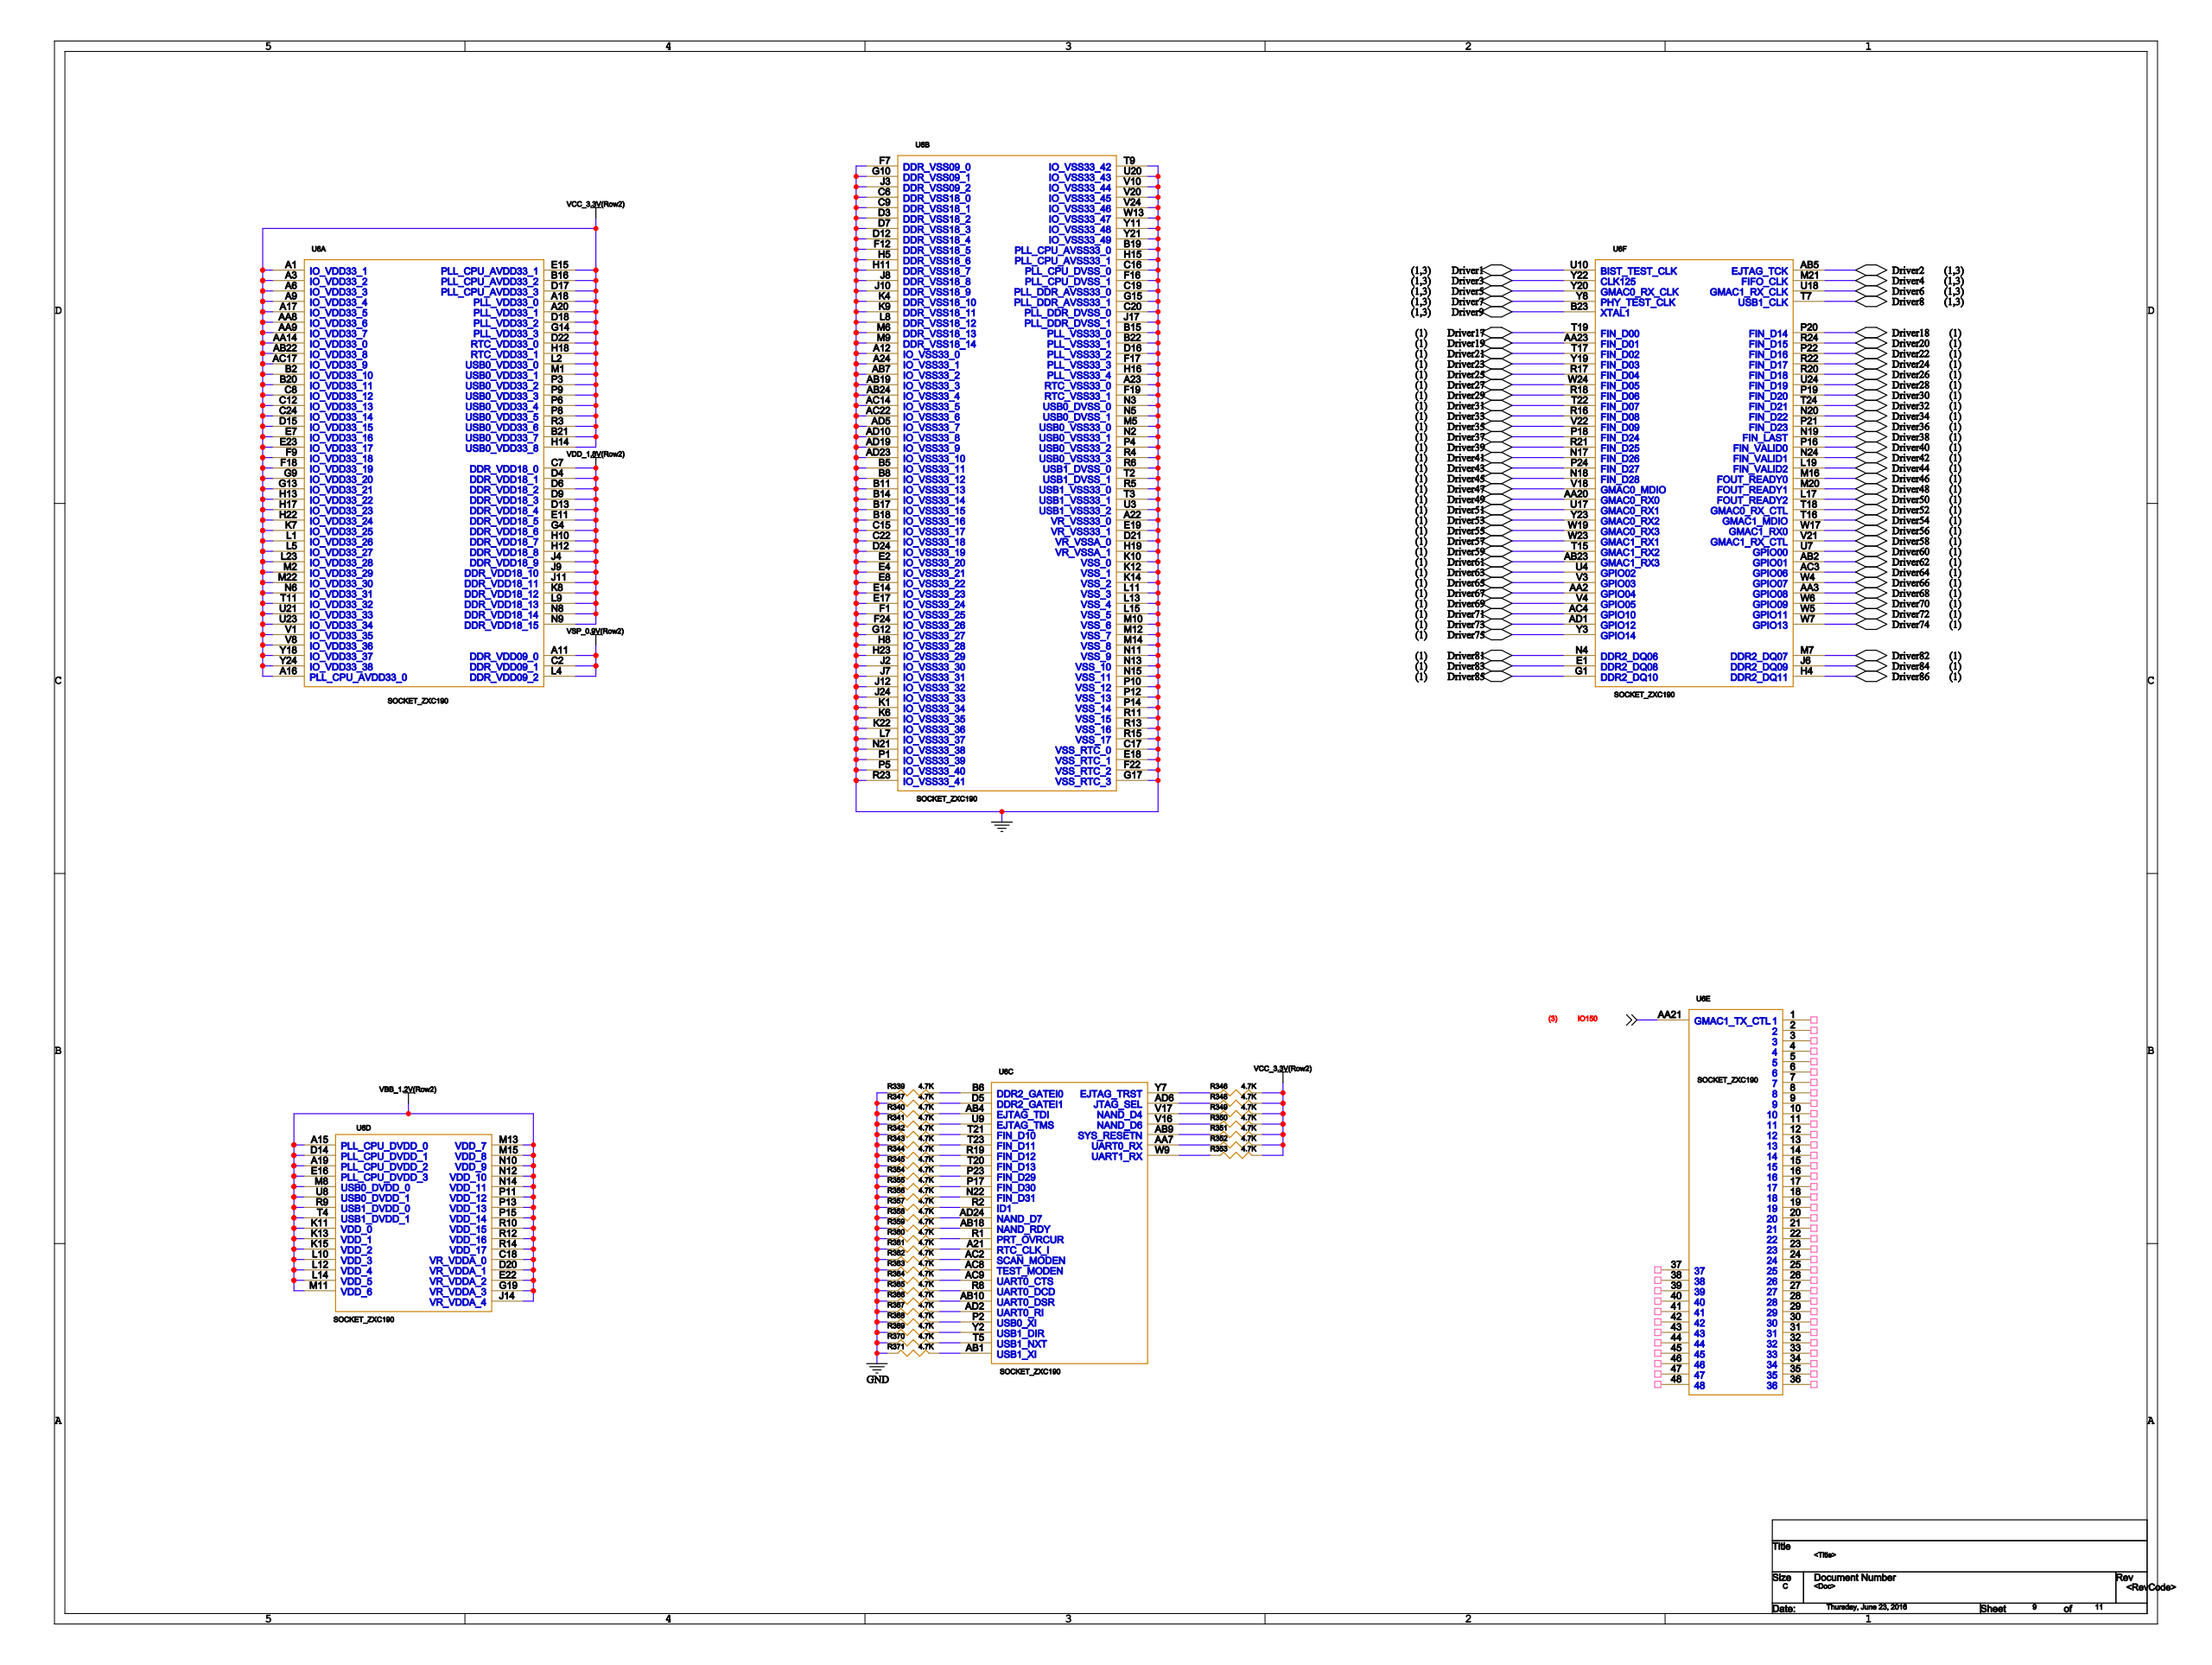Circuit board | Cadence Allegro | 531 parts | 624 nets | one sheet of the schematic
Parts on this sheet (reference | value | footprint):
R339 | 4.7K | R0805
R340 | 4.7K | R0805
R341 | 4.7K | R0805
R342 | 4.7K | R0805
R343 | 4.7K | R0805
R344 | 4.7K | R0805
R345 | 4.7K | R0805
R346 | 4.7K | R0805
R347 | 4.7K | R0805
R348 | 4.7K | R0805
R349 | 4.7K | R0805
R350 | 4.7K | R0805
R351 | 4.7K | R0805
R352 | 4.7K | R0805
R353 | 4.7K | R0805
R354 | 4.7K | R0805
R355 | 4.7K | R0805
R356 | 4.7K | R0805
R357 | 4.7K | R0805
R358 | 4.7K | R0805
R359 | 4.7K | R0805
R360 | 4.7K | R0805
R361 | 4.7K | R0805
R362 | 4.7K | R0805
R363 | 4.7K | R0805
R364 | 4.7K | R0805
R365 | 4.7K | R0805
R366 | 4.7K | R0805
R367 | 4.7K | R0805
R368 | 4.7K | R0805
R369 | 4.7K | R0805
R370 | 4.7K | R0805
R371 | 4.7K | R0805
U3 | SOCKET_ZXC190 | BGA-576
U4 | SOCKET_ZXC190 | BGA-576
U6 | SOCKET_ZXC190 | BGA-576
U10 | SOCKET_ZXC190 | BGA-576
Nets of these parts (net: part-pin ...):
GND: R339-1 R340-1 R341-1 R342-1 R343-1 R344-1 R345-1 R347-1 R354-1 R355-1 R356-1 R357-1 R358-1 R359-1 R360-1 R361-1 R362-1 R363-1 R364-1 R365-1 R366-1 R367-1 R368-1 R369-1 R370-1 R371-1 U3-A12 U3-A22 U3-A23 U3-A24 U3-AB7 U3-AB19 U3-AB24 U3-AC14 U3-AC22 U3-AD5 U3-AD10 U3-AD19 U3-AD23 U3-B5 U3-B8 U3-B11 U3-B14 U3-B15 U3-B17 U3-B18 U3-B19 U3-B22 U3-C6 U3-C9 U3-C15 U3-C16 U3-C17 U3-C19 U3-C20 U3-C22 U3-D3 U3-D7 U3-D12 U3-D16 U3-D21 U3-D24 U3-E2 U3-E4 U3-E8 U3-E14 U3-E17 U3-E18 U3-E19 U3-F1 U3-F7 U3-F12 U3-F16 U3-F17 U3-F19 U3-F22 U3-F24 U3-G10 U3-G12 U3-G15 U3-G17 U3-H5 U3-H8 U3-H11 U3-H15 U3-H16 U3-H19 U3-H23 U3-J2 U3-J3 U3-J7 U3-J8 U3-J10 U3-J12 U3-J17 U3-J24 U3-K1 U3-K4 U3-K6 U3-K9 U3-K10 U3-K12 U3-K14 U3-K22 U3-L7 U3-L8 U3-L11 U3-L13 U3-L15 U3-M5 U3-M6 U3-M9 U3-M10 U3-M12 U3-M14 U3-N2 U3-N3 U3-N5 U3-N11 U3-N13 U3-N15 U3-N21 U3-P1 U3-P4 U3-P5 U3-P10 U3-P12 U3-P14 U3-R4 U3-R5 U3-R6 U3-R11 U3-R13 U3-R15 U3-R23 U3-T2 U3-T3 U3-T9 U3-U3 U3-U20 U3-V10 U3-V20 U3-V24 U3-W13 U3-Y11 U3-Y21 U4-A12 U4-A22 U4-A23 U4-A24 U4-AB7 U4-AB19 U4-AB24 U4-AC14 U4-AC22 U4-AD5 U4-AD10 U4-AD19 U4-AD23 U4-B5 U4-B8 U4-B11 U4-B14 U4-B15 U4-B17 U4-B18 U4-B19 U4-B22 U4-C6 U4-C9 U4-C15 U4-C16 U4-C17 U4-C19 U4-C20 U4-C22 U4-D3 U4-D7 U4-D12 U4-D16 U4-D21 U4-D24 U4-E2 U4-E4 U4-E8 U4-E14 U4-E17 U4-E18 U4-E19 U4-F1 U4-F7 U4-F12 U4-F16 U4-F17 U4-F19 U4-F22 U4-F24 U4-G10 U4-G12 U4-G15 U4-G17 U4-H5 U4-H8 U4-H11 U4-H15 U4-H16 U4-H19 U4-H23 U4-J2 U4-J3 U4-J7 U4-J8 U4-J10 U4-J12 U4-J17 U4-J24 U4-K1 U4-K4 U4-K6 U4-K9 U4-K10 U4-K12 U4-K14 U4-K22 U4-L7 U4-L8 U4-L11 U4-L13 U4-L15 U4-M5 U4-M6 U4-M9 U4-M10 U4-M12 U4-M14 U4-N2 U4-N3 U4-N5 U4-N11 U4-N13 U4-N15 U4-N21 U4-P1 U4-P4 U4-P5 U4-P10 U4-P12 U4-P14 U4-R4 U4-R5 U4-R6 U4-R11 U4-R13 U4-R15 U4-R23 U4-T2 U4-T3 U4-T9 U4-U3 U4-U20 U4-V10 U4-V20 U4-V24 U4-W13 U4-Y11 U4-Y21 U6-A12 U6-A22 U6-A23 U6-A24 U6-AB7 U6-AB19 U6-AB24 U6-AC14 U6-AC22 U6-AD5 U6-AD10 U6-AD19 U6-AD23 U6-B5 U6-B8 U6-B11 U6-B14 U6-B15 U6-B17 U6-B18 U6-B19 U6-B22 U6-C6 U6-C9 U6-C15 U6-C16 U6-C17 U6-C19 U6-C20 U6-C22 U6-D3 U6-D7 U6-D12 U6-D16 U6-D21 U6-D24 U6-E2 U6-E4 U6-E8 U6-E14 U6-E17 U6-E18 U6-E19 U6-F1 U6-F7 U6-F12 U6-F16 U6-F17 U6-F19 U6-F22 U6-F24 U6-G10 U6-G12 U6-G15 U6-G17 U6-H5 U6-H8 U6-H11 U6-H15 U6-H16 U6-H19 U6-H23 U6-J2 U6-J3 U6-J7 U6-J8 U6-J10 U6-J12 U6-J17 U6-J24 U6-K1 U6-K4 U6-K6 U6-K9 U6-K10 U6-K12 U6-K14 U6-K22 U6-L7 U6-L8 U6-L11 U6-L13 U6-L15 U6-M5 U6-M6 U6-M9 U6-M10 U6-M12 U6-M14 U6-N2 U6-N3 U6-N5 U6-N11 U6-N13 U6-N15 U6-N21 U6-P1 U6-P4 U6-P5 U6-P10 U6-P12 U6-P14 U6-R4 U6-R5 U6-R6 U6-R11 U6-R13 U6-R15 U6-R23 U6-T2 U6-T3 U6-T9 U6-U3 U6-U20 U6-V10 U6-V20 U6-V24 U6-W13 U6-Y11 U6-Y21 U10-A12 U10-A22 U10-A23 U10-A24 U10-AB7 U10-AB19 U10-AB24 U10-AC14 U10-AC22 U10-AD5 U10-AD10 U10-AD19 U10-AD23 U10-B5 U10-B8 U10-B11 U10-B14 U10-B15 U10-B17 U10-B18 U10-B19 U10-B22 U10-C6 U10-C9 U10-C15 U10-C16 U10-C17 U10-C19 U10-C20 U10-C22 U10-D3 U10-D7 U10-D12 U10-D16 U10-D21 U10-D24 U10-E2 U10-E4 U10-E8 U10-E14 U10-E17 U10-E18 U10-E19 U10-F1 U10-F7 U10-F12 U10-F16 U10-F17 U10-F19 U10-F22 U10-F24 U10-G10 U10-G12 U10-G15 U10-G17 U10-H5 U10-H8 U10-H11 U10-H15 U10-H16 U10-H19 U10-H23 U10-J2 U10-J3 U10-J7 U10-J8 U10-J10 U10-J12 U10-J17 U10-J24 U10-K1 U10-K4 U10-K6 U10-K9 U10-K10 U10-K12 U10-K14 U10-K22 U10-L7 U10-L8 U10-L11 U10-L13 U10-L15 U10-M5 U10-M6 U10-M9 U10-M10 U10-M12 U10-M14 U10-N2 U10-N3 U10-N5 U10-N11 U10-N13 U10-N15 U10-N21 U10-P1 U10-P4 U10-P5 U10-P10 U10-P12 U10-P14 U10-R4 U10-R5 U10-R6 U10-R11 U10-R13 U10-R15 U10-R23 U10-T2 U10-T3 U10-T9 U10-U3 U10-U20 U10-V10 U10-V20 U10-V24 U10-W13 U10-Y11 U10-Y21
VCC_3.3V(ROW2): R346-2 R348-2 R349-2 R350-2 R351-2 R352-2 R353-2 U6-A1 U6-A3 U6-A6 U6-A9 U6-A16 U6-A17 U6-A18 U6-A20 U6-AA8 U6-AA9 U6-AA14 U6-AB22 U6-AC17 U6-B2 U6-B16 U6-B20 U6-B21 U6-C8 U6-C12 U6-C24 U6-D15 U6-D17 U6-D18 U6-D22 U6-E7 U6-E15 U6-E23 U6-F9 U6-F18 U6-G9 U6-G13 U6-G14 U6-H13 U6-H14 U6-H17 U6-H18 U6-H22 U6-K7 U6-L1 U6-L2 U6-L5 U6-L23 U6-M1 U6-M2 U6-M22 U6-N6 U6-P3 U6-P6 U6-P8 U6-P9 U6-R3 U6-T11 U6-U21 U6-U23 U6-V1 U6-V8 U6-Y18 U6-Y24 U10-A1 U10-A3 U10-A6 U10-A9 U10-A16 U10-A17 U10-A18 U10-A20 U10-AA8 U10-AA9 U10-AA14 U10-AB22 U10-AC17 U10-B2 U10-B16 U10-B20 U10-B21 U10-C8 U10-C12 U10-C24 U10-D15 U10-D17 U10-D18 U10-D22 U10-E7 U10-E15 U10-E23 U10-F9 U10-F18 U10-G9 U10-G13 U10-G14 U10-H13 U10-H14 U10-H17 U10-H18 U10-H22 U10-K7 U10-L1 U10-L2 U10-L5 U10-L23 U10-M1 U10-M2 U10-M22 U10-N6 U10-P3 U10-P6 U10-P8 U10-P9 U10-R3 U10-T11 U10-U21 U10-U23 U10-V1 U10-V8 U10-Y18 U10-Y24
N8556432: R339-2 U6-B6
N8556424: R340-2 U6-AB4
N8556420: R341-2 U6-U9
N8556416: R342-2 U6-T21
N8556412: R343-2 U6-T23
N8556408: R344-2 U6-R19
N8556464: R345-2 U6-T20
N8556856: R346-1 U6-Y7
N8556428: R347-2 U6-D5
N8556892: R348-1 U6-AD6
N8557036: R349-1 U6-V17
N8557040: R350-1 U6-V16
N8557064: R351-1 U6-AB9
N8557044: R352-1 U6-AA7
N8556388: R353-1 U6-W9
N8556460: R354-2 U6-P23
N8556456: R355-2 U6-P17
N8556452: R356-2 U6-N22
N8556448: R357-2 U6-R2
N8556444: R358-2 U6-AD24
N8556440: R359-2 U6-AB18
N8556436: R360-2 U6-R1
N8556492: R361-2 U6-A21
N8556488: R362-2 U6-AC2
N8556484: R363-2 U6-AC8
N8556480: R364-2 U6-AC9
N8556928: R365-2 U6-R8
N8556476: R366-2 U6-AB10
N8556472: R367-2 U6-AD2
N8556468: R368-2 U6-P2
N8556504: R369-2 U6-Y2
N8556500: R370-2 U6-T5
N8556496: R371-2 U6-AB1
IO150: U6-AA21